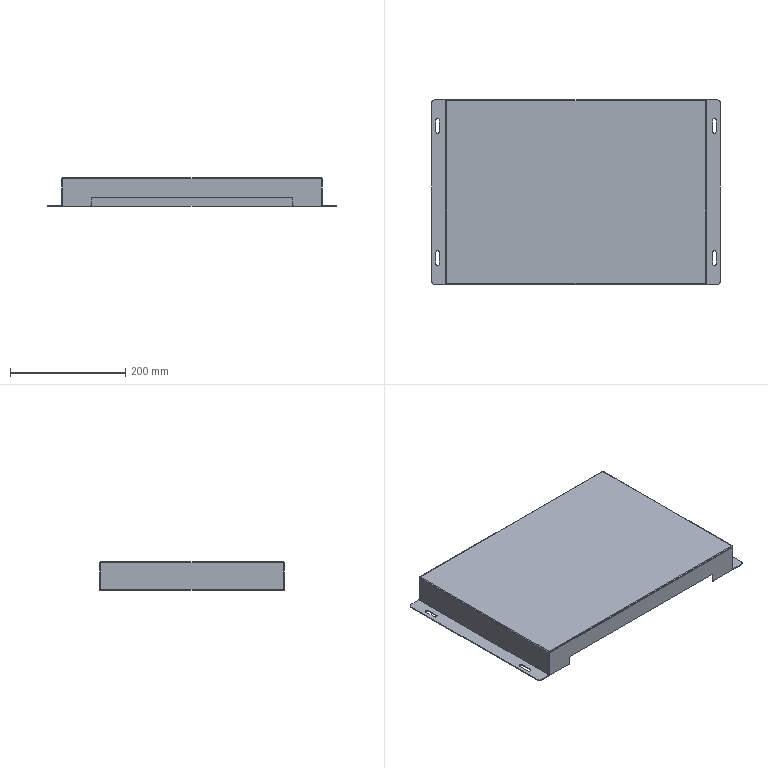Part | STEP file | NX21002-02-MA-J-002 | 1 solid | 54 faces | box 500 x 320 x 50 mm | volume 341606 mm3 | plane 26 | cylinder 24 | sphere 4 | commonest cylinder face diameters 4 x12 6 x8 10 x4